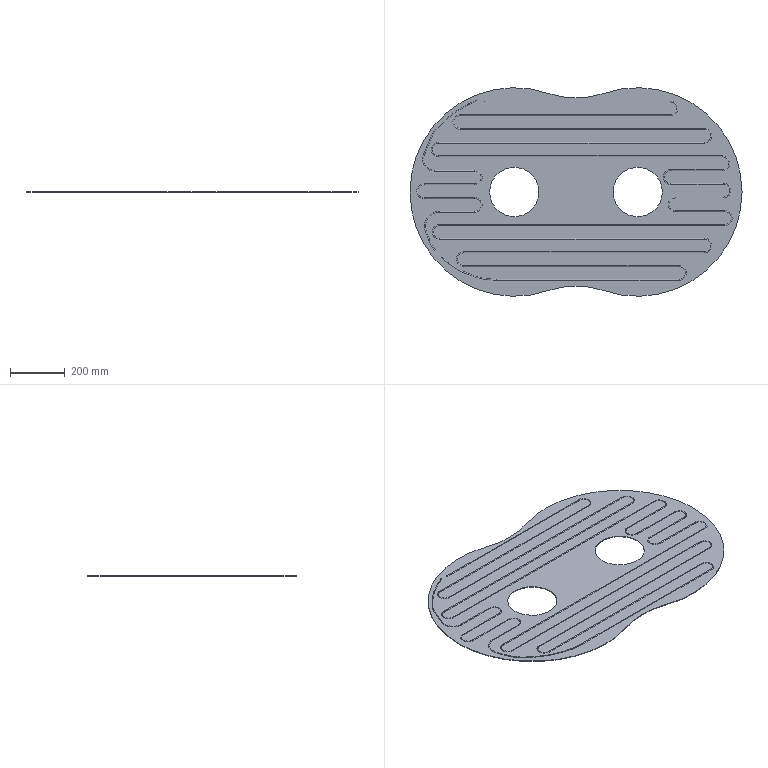Part | NX | 3 solids | 56 faces | box 1210 x 760 x 3.5 mm | volume 1542690 mm3 | cylinder 29 | torus 21 | plane 6 | commonest cylinder face diameters 3 x23 180 x2 640 x2 760 x2
STEP:
#1=CARTESIAN_POINT('',(2647.074,604.738,0.));
#2=VERTEX_POINT('',#1);
#3=CARTESIAN_POINT('',(2647.074,-114.931,0.));
#4=VERTEX_POINT('',#3);
#5=CARTESIAN_POINT('',(2524.931,244.903,0.));
#6=DIRECTION('',(0.,0.,1.));
#7=DIRECTION('',(1.,0.,0.));
#8=AXIS2_PLACEMENT_3D('',#5,#6,#7);
#9=CIRCLE('',#8,380.);
#10=EDGE_CURVE('',#2,#4,#9,.T.);
#11=ORIENTED_EDGE('',*,*,#10,.T.);
#12=CARTESIAN_POINT('',(2647.074,-114.931,2.));
#13=VERTEX_POINT('',#12);
#14=CARTESIAN_POINT('',(2647.074,-114.931,2.));
#15=DIRECTION('',(0.,0.,-1.));
#16=VECTOR('',#15,1.);
#17=LINE('',#14,#16);
#18=EDGE_CURVE('',#13,#4,#17,.T.);
#19=ORIENTED_EDGE('',*,*,#18,.F.);
#20=CARTESIAN_POINT('',(2647.074,604.738,2.));
#21=VERTEX_POINT('',#20);
#22=CARTESIAN_POINT('',(2524.931,244.903,2.));
#23=DIRECTION('',(0.,0.,1.));
#24=DIRECTION('',(1.,0.,0.));
#25=AXIS2_PLACEMENT_3D('',#22,#23,#24);
#26=CIRCLE('',#25,380.);
#27=EDGE_CURVE('',#21,#13,#26,.T.);
#28=ORIENTED_EDGE('',*,*,#27,.F.);
#29=CARTESIAN_POINT('',(2647.074,604.738,2.));
#30=DIRECTION('',(0.,0.,-1.));
#31=VECTOR('',#30,1.);
#32=LINE('',#29,#31);
#33=EDGE_CURVE('',#21,#2,#32,.T.);
#34=ORIENTED_EDGE('',*,*,#33,.T.);
#35=EDGE_LOOP('',(#11,#19,#28,#34));
#36=FACE_OUTER_BOUND('',#35,.T.);
#37=CARTESIAN_POINT('',(2524.931,244.903,2.));
#38=DIRECTION('',(0.,0.,-1.));
#39=DIRECTION('',(-1.,0.,0.));
#40=AXIS2_PLACEMENT_3D('',#37,#38,#39);
#41=CYLINDRICAL_SURFACE('',#40,380.);
#42=ADVANCED_FACE('',(#36),#41,.T.);
#43=CARTESIAN_POINT('',(2852.788,-114.931,0.));
#44=VERTEX_POINT('',#43);
#45=CARTESIAN_POINT('',(2749.931,-417.95,0.));
#46=DIRECTION('',(0.,0.,-1.));
#47=DIRECTION('',(1.,0.,0.));
#48=AXIS2_PLACEMENT_3D('',#45,#46,#47);
#49=CIRCLE('',#48,320.);
#50=EDGE_CURVE('',#4,#44,#49,.T.);
#51=ORIENTED_EDGE('',*,*,#50,.T.);
#52=CARTESIAN_POINT('',(2852.788,-114.931,2.));
#53=VERTEX_POINT('',#52);
#54=CARTESIAN_POINT('',(2852.788,-114.931,2.));
#55=DIRECTION('',(0.,0.,-1.));
#56=VECTOR('',#55,1.);
#57=LINE('',#54,#56);
#58=EDGE_CURVE('',#53,#44,#57,.T.);
#59=ORIENTED_EDGE('',*,*,#58,.F.);
#60=CARTESIAN_POINT('',(2749.931,-417.95,2.));
#61=DIRECTION('',(0.,0.,-1.));
#62=DIRECTION('',(1.,0.,0.));
#63=AXIS2_PLACEMENT_3D('',#60,#61,#62);
#64=CIRCLE('',#63,320.);
#65=EDGE_CURVE('',#13,#53,#64,.T.);
#66=ORIENTED_EDGE('',*,*,#65,.F.);
#67=ORIENTED_EDGE('',*,*,#18,.T.);
#68=EDGE_LOOP('',(#51,#59,#66,#67));
#69=FACE_OUTER_BOUND('',#68,.T.);
#70=CARTESIAN_POINT('',(2749.931,-417.95,2.));
#71=DIRECTION('',(0.,0.,-1.));
#72=DIRECTION('',(-1.,0.,0.));
#73=AXIS2_PLACEMENT_3D('',#70,#71,#72);
#74=CYLINDRICAL_SURFACE('',#73,320.);
#75=ADVANCED_FACE('',(#69),#74,.F.);
#76=CARTESIAN_POINT('',(2852.788,604.738,0.));
#77=VERTEX_POINT('',#76);
#78=CARTESIAN_POINT('',(2974.931,244.903,0.));
#79=DIRECTION('',(0.,0.,1.));
#80=DIRECTION('',(1.,0.,0.));
#81=AXIS2_PLACEMENT_3D('',#78,#79,#80);
#82=CIRCLE('',#81,380.);
#83=EDGE_CURVE('',#44,#77,#82,.T.);
#84=ORIENTED_EDGE('',*,*,#83,.T.);
#85=CARTESIAN_POINT('',(2852.788,604.738,2.));
#86=VERTEX_POINT('',#85);
#87=CARTESIAN_POINT('',(2852.788,604.738,2.));
#88=DIRECTION('',(0.,0.,-1.));
#89=VECTOR('',#88,1.);
#90=LINE('',#87,#89);
#91=EDGE_CURVE('',#86,#77,#90,.T.);
#92=ORIENTED_EDGE('',*,*,#91,.F.);
#93=CARTESIAN_POINT('',(2974.931,244.903,2.));
#94=DIRECTION('',(0.,0.,1.));
#95=DIRECTION('',(1.,0.,0.));
#96=AXIS2_PLACEMENT_3D('',#93,#94,#95);
#97=CIRCLE('',#96,380.);
#98=EDGE_CURVE('',#53,#86,#97,.T.);
#99=ORIENTED_EDGE('',*,*,#98,.F.);
#100=ORIENTED_EDGE('',*,*,#58,.T.);
#101=EDGE_LOOP('',(#84,#92,#99,#100));
#102=FACE_OUTER_BOUND('',#101,.T.);
#103=CARTESIAN_POINT('',(2974.931,244.903,2.));
#104=DIRECTION('',(0.,0.,-1.));
#105=DIRECTION('',(-1.,0.,0.));
#106=AXIS2_PLACEMENT_3D('',#103,#104,#105);
#107=CYLINDRICAL_SURFACE('',#106,380.);
#108=ADVANCED_FACE('',(#102),#107,.T.);
#109=CARTESIAN_POINT('',(2614.931,244.903,2.));
#110=VERTEX_POINT('',#109);
#111=CARTESIAN_POINT('',(2524.931,244.903,2.));
#112=DIRECTION('',(0.,0.,1.));
#113=DIRECTION('',(1.,0.,0.));
#114=AXIS2_PLACEMENT_3D('',#111,#112,#113);
#115=CIRCLE('',#114,90.);
#116=EDGE_CURVE('',#110,#110,#115,.T.);
#117=ORIENTED_EDGE('',*,*,#116,.T.);
#118=EDGE_LOOP('',(#117));
#119=FACE_BOUND('',#118,.T.);
#120=CARTESIAN_POINT('',(2614.931,244.903,0.));
#121=VERTEX_POINT('',#120);
#122=CARTESIAN_POINT('',(2524.931,244.903,0.));
#123=DIRECTION('',(0.,0.,1.));
#124=DIRECTION('',(1.,0.,0.));
#125=AXIS2_PLACEMENT_3D('',#122,#123,#124);
#126=CIRCLE('',#125,90.);
#127=EDGE_CURVE('',#121,#121,#126,.T.);
#128=ORIENTED_EDGE('',*,*,#127,.F.);
#129=EDGE_LOOP('',(#128));
#130=FACE_BOUND('',#129,.T.);
#131=CARTESIAN_POINT('',(2524.931,244.903,2.));
#132=DIRECTION('',(0.,0.,-1.));
#133=DIRECTION('',(-1.,0.,0.));
#134=AXIS2_PLACEMENT_3D('',#131,#132,#133);
#135=CYLINDRICAL_SURFACE('',#134,90.);
#136=ADVANCED_FACE('',(#119,#130),#135,.F.);
#137=CARTESIAN_POINT('',(2749.931,907.757,0.));
#138=DIRECTION('',(0.,0.,-1.));
#139=DIRECTION('',(1.,0.,0.));
#140=AXIS2_PLACEMENT_3D('',#137,#138,#139);
#141=CIRCLE('',#140,320.);
#142=EDGE_CURVE('',#77,#2,#141,.T.);
#143=ORIENTED_EDGE('',*,*,#142,.T.);
#144=ORIENTED_EDGE('',*,*,#33,.F.);
#145=CARTESIAN_POINT('',(2749.931,907.757,2.));
#146=DIRECTION('',(0.,0.,-1.));
#147=DIRECTION('',(1.,0.,0.));
#148=AXIS2_PLACEMENT_3D('',#145,#146,#147);
#149=CIRCLE('',#148,320.);
#150=EDGE_CURVE('',#86,#21,#149,.T.);
#151=ORIENTED_EDGE('',*,*,#150,.F.);
#152=ORIENTED_EDGE('',*,*,#91,.T.);
#153=EDGE_LOOP('',(#143,#144,#151,#152));
#154=FACE_OUTER_BOUND('',#153,.T.);
#155=CARTESIAN_POINT('',(2749.931,907.757,2.));
#156=DIRECTION('',(0.,0.,-1.));
#157=DIRECTION('',(-1.,0.,0.));
#158=AXIS2_PLACEMENT_3D('',#155,#156,#157);
#159=CYLINDRICAL_SURFACE('',#158,320.);
#160=ADVANCED_FACE('',(#154),#159,.F.);
#161=CARTESIAN_POINT('',(3064.931,244.903,2.));
#162=VERTEX_POINT('',#161);
#163=CARTESIAN_POINT('',(2974.931,244.903,2.));
#164=DIRECTION('',(0.,0.,1.));
#165=DIRECTION('',(1.,0.,0.));
#166=AXIS2_PLACEMENT_3D('',#163,#164,#165);
#167=CIRCLE('',#166,90.);
#168=EDGE_CURVE('',#162,#162,#167,.T.);
#169=ORIENTED_EDGE('',*,*,#168,.T.);
#170=EDGE_LOOP('',(#169));
#171=FACE_BOUND('',#170,.T.);
#172=CARTESIAN_POINT('',(3064.931,244.903,0.));
#173=VERTEX_POINT('',#172);
#174=CARTESIAN_POINT('',(2974.931,244.903,0.));
#175=DIRECTION('',(0.,0.,1.));
#176=DIRECTION('',(1.,0.,0.));
#177=AXIS2_PLACEMENT_3D('',#174,#175,#176);
#178=CIRCLE('',#177,90.);
#179=EDGE_CURVE('',#173,#173,#178,.T.);
#180=ORIENTED_EDGE('',*,*,#179,.F.);
#181=EDGE_LOOP('',(#180));
#182=FACE_BOUND('',#181,.T.);
#183=CARTESIAN_POINT('',(2974.931,244.903,2.));
#184=DIRECTION('',(0.,0.,-1.));
#185=DIRECTION('',(-1.,0.,0.));
#186=AXIS2_PLACEMENT_3D('',#183,#184,#185);
#187=CYLINDRICAL_SURFACE('',#186,90.);
#188=ADVANCED_FACE('',(#171,#182),#187,.F.);
#189=ORIENTED_EDGE('',*,*,#27,.T.);
#190=ORIENTED_EDGE('',*,*,#65,.T.);
#191=ORIENTED_EDGE('',*,*,#98,.T.);
#192=ORIENTED_EDGE('',*,*,#150,.T.);
#193=EDGE_LOOP('',(#189,#190,#191,#192));
#194=FACE_BOUND('',#193,.T.);
#195=ORIENTED_EDGE('',*,*,#116,.F.);
#196=EDGE_LOOP('',(#195));
#197=FACE_BOUND('',#196,.T.);
#198=ORIENTED_EDGE('',*,*,#168,.F.);
#199=EDGE_LOOP('',(#198));
#200=FACE_BOUND('',#199,.T.);
#201=CARTESIAN_POINT('',(2637.431,-86.523,2.));
#202=DIRECTION('',(0.,0.,1.));
#203=DIRECTION('',(1.,0.,0.));
#204=AXIS2_PLACEMENT_3D('',#201,#202,#203);
#205=PLANE('',#204);
#206=ADVANCED_FACE('',(#194,#197,#200),#205,.T.);
#207=ORIENTED_EDGE('',*,*,#10,.F.);
#208=ORIENTED_EDGE('',*,*,#142,.F.);
#209=ORIENTED_EDGE('',*,*,#83,.F.);
#210=ORIENTED_EDGE('',*,*,#50,.F.);
#211=EDGE_LOOP('',(#207,#208,#209,#210));
#212=FACE_BOUND('',#211,.T.);
#213=ORIENTED_EDGE('',*,*,#127,.T.);
#214=EDGE_LOOP('',(#213));
#215=FACE_BOUND('',#214,.T.);
#216=ORIENTED_EDGE('',*,*,#179,.T.);
#217=EDGE_LOOP('',(#216));
#218=FACE_BOUND('',#217,.T.);
#219=CARTESIAN_POINT('',(2637.431,-86.523,0.));
#220=DIRECTION('',(0.,0.,1.));
#221=DIRECTION('',(1.,0.,0.));
#222=AXIS2_PLACEMENT_3D('',#219,#220,#221);
#223=PLANE('',#222);
#224=ADVANCED_FACE('',(#212,#215,#218),#223,.F.);
#225=CLOSED_SHELL('',(#42,#75,#108,#136,#160,#188,#206,#224));
#226=MANIFOLD_SOLID_BREP('',#225);
#227=CARTESIAN_POINT('',(2239.156,471.609,2.));
#228=VERTEX_POINT('',#227);
#229=CARTESIAN_POINT('',(2238.018,472.586,2.));
#230=DIRECTION('',(-0.6509,-0.7592,0.));
#231=DIRECTION('',(0.7592,-0.6509,0.));
#232=AXIS2_PLACEMENT_3D('',#229,#230,#231);
#233=CIRCLE('',#232,1.5);
#234=EDGE_CURVE('',#228,#228,#233,.T.);
#235=ORIENTED_EDGE('',*,*,#234,.T.);
#236=EDGE_LOOP('',(#235));
#237=FACE_BOUND('',#236,.T.);
#238=CARTESIAN_POINT('',(2232.864,464.27,2.));
#239=VERTEX_POINT('',#238);
#240=CARTESIAN_POINT('',(2231.725,465.246,2.));
#241=DIRECTION('',(-0.6509,-0.7592,0.));
#242=DIRECTION('',(0.7592,-0.6509,0.));
#243=AXIS2_PLACEMENT_3D('',#240,#241,#242);
#244=CIRCLE('',#243,1.5);
#245=EDGE_CURVE('',#239,#239,#244,.T.);
#246=ORIENTED_EDGE('',*,*,#245,.F.);
#247=EDGE_LOOP('',(#246));
#248=FACE_BOUND('',#247,.T.);
#249=CARTESIAN_POINT('',(2238.018,472.586,2.));
#250=DIRECTION('',(-0.6509,-0.7592,0.));
#251=DIRECTION('',(0.7592,-0.6509,0.));
#252=AXIS2_PLACEMENT_3D('',#249,#250,#251);
#253=CYLINDRICAL_SURFACE('',#252,1.5);
#254=ADVANCED_FACE('',(#237,#248),#253,.T.);
#255=CARTESIAN_POINT('',(2359.815,563.182,2.));
#256=VERTEX_POINT('',#255);
#257=CARTESIAN_POINT('',(2359.181,564.541,2.));
#258=DIRECTION('',(-0.9063,-0.4226,0.));
#259=DIRECTION('',(0.4226,-0.9063,0.));
#260=AXIS2_PLACEMENT_3D('',#257,#258,#259);
#261=CIRCLE('',#260,1.5);
#262=EDGE_CURVE('',#256,#256,#261,.T.);
#263=ORIENTED_EDGE('',*,*,#262,.T.);
#264=EDGE_LOOP('',(#263));
#265=FACE_BOUND('',#264,.T.);
#266=ORIENTED_EDGE('',*,*,#234,.F.);
#267=EDGE_LOOP('',(#266));
#268=FACE_BOUND('',#267,.T.);
#269=CARTESIAN_POINT('',(2511.324,238.271,2.));
#270=DIRECTION('',(0.,0.,1.));
#271=DIRECTION('',(1.,0.,0.));
#272=AXIS2_PLACEMENT_3D('',#269,#270,#271);
#273=TOROIDAL_SURFACE('',#272,360.,1.5);
#274=ADVANCED_FACE('',(#265,#268),#273,.T.);
#275=ORIENTED_EDGE('',*,*,#262,.F.);
#276=EDGE_LOOP('',(#275));
#277=FACE_BOUND('',#276,.T.);
#278=CARTESIAN_POINT('',(2388.99,576.786,2.));
#279=VERTEX_POINT('',#278);
#280=CARTESIAN_POINT('',(2388.356,578.146,2.));
#281=DIRECTION('',(-0.9063,-0.4226,0.));
#282=DIRECTION('',(0.4226,-0.9063,0.));
#283=AXIS2_PLACEMENT_3D('',#280,#281,#282);
#284=CIRCLE('',#283,1.5);
#285=EDGE_CURVE('',#279,#279,#284,.T.);
#286=ORIENTED_EDGE('',*,*,#285,.T.);
#287=EDGE_LOOP('',(#286));
#288=FACE_BOUND('',#287,.T.);
#289=CARTESIAN_POINT('',(2359.181,564.541,2.));
#290=DIRECTION('',(0.9063,0.4226,0.));
#291=DIRECTION('',(-0.4226,0.9063,0.));
#292=AXIS2_PLACEMENT_3D('',#289,#290,#291);
#293=CYLINDRICAL_SURFACE('',#292,1.5);
#294=ADVANCED_FACE('',(#277,#288),#293,.T.);
#295=ORIENTED_EDGE('',*,*,#245,.T.);
#296=EDGE_LOOP('',(#295));
#297=FACE_OUTER_BOUND('',#296,.T.);
#298=CARTESIAN_POINT('',(2231.725,465.246,2.));
#299=DIRECTION('',(-0.6509,-0.7592,0.));
#300=DIRECTION('',(0.7592,-0.6509,0.));
#301=AXIS2_PLACEMENT_3D('',#298,#299,#300);
#302=PLANE('',#301);
#303=ADVANCED_FACE('',(#297),#302,.T.);
#304=ORIENTED_EDGE('',*,*,#285,.F.);
#305=EDGE_LOOP('',(#304));
#306=FACE_OUTER_BOUND('',#305,.T.);
#307=CARTESIAN_POINT('',(2388.356,578.146,2.));
#308=DIRECTION('',(-0.9063,-0.4226,0.));
#309=DIRECTION('',(0.4226,-0.9063,0.));
#310=AXIS2_PLACEMENT_3D('',#307,#308,#309);
#311=PLANE('',#310);
#312=ADVANCED_FACE('',(#306),#311,.F.);
#313=CLOSED_SHELL('',(#254,#274,#294,#303,#312));
#314=MANIFOLD_SOLID_BREP('',#313);
#315=CARTESIAN_POINT('',(3094.34,573.238,2.));
#316=VERTEX_POINT('',#315);
#317=CARTESIAN_POINT('',(3094.34,574.738,2.));
#318=DIRECTION('',(-1.,0.,0.));
#319=DIRECTION('',(0.,-1.,0.));
#320=AXIS2_PLACEMENT_3D('',#317,#318,#319);
#321=CIRCLE('',#320,1.5);
#322=EDGE_CURVE('',#316,#316,#321,.T.);
#323=ORIENTED_EDGE('',*,*,#322,.T.);
#324=EDGE_LOOP('',(#323));
#325=FACE_BOUND('',#324,.T.);
#326=CARTESIAN_POINT('',(2415.256,573.238,2.));
#327=VERTEX_POINT('',#326);
#328=CARTESIAN_POINT('',(2415.256,574.738,2.));
#329=DIRECTION('',(-1.,0.,0.));
#330=DIRECTION('',(0.,-1.,0.));
#331=AXIS2_PLACEMENT_3D('',#328,#329,#330);
#332=CIRCLE('',#331,1.5);
#333=EDGE_CURVE('',#327,#327,#332,.T.);
#334=ORIENTED_EDGE('',*,*,#333,.F.);
#335=EDGE_LOOP('',(#334));
#336=FACE_BOUND('',#335,.T.);
#337=CARTESIAN_POINT('',(3094.34,574.738,2.));
#338=DIRECTION('',(-1.,0.,0.));
#339=DIRECTION('',(0.,0.,1.));
#340=AXIS2_PLACEMENT_3D('',#337,#338,#339);
#341=CYLINDRICAL_SURFACE('',#340,1.5);
#342=ADVANCED_FACE('',(#325,#336),#341,.T.);
#343=CARTESIAN_POINT('',(3094.34,526.238,2.));
#344=VERTEX_POINT('',#343);
#345=CARTESIAN_POINT('',(3094.34,524.738,2.));
#346=DIRECTION('',(1.,0.,0.));
#347=DIRECTION('',(0.,1.,0.));
#348=AXIS2_PLACEMENT_3D('',#345,#346,#347);
#349=CIRCLE('',#348,1.5);
#350=EDGE_CURVE('',#344,#344,#349,.T.);
#351=ORIENTED_EDGE('',*,*,#350,.T.);
#352=EDGE_LOOP('',(#351));
#353=FACE_BOUND('',#352,.T.);
#354=ORIENTED_EDGE('',*,*,#322,.F.);
#355=EDGE_LOOP('',(#354));
#356=FACE_BOUND('',#355,.T.);
#357=CARTESIAN_POINT('',(3094.34,549.738,2.));
#358=DIRECTION('',(0.,0.,1.));
#359=DIRECTION('',(1.,0.,0.));
#360=AXIS2_PLACEMENT_3D('',#357,#358,#359);
#361=TOROIDAL_SURFACE('',#360,25.,1.5);
#362=ADVANCED_FACE('',(#353,#356),#361,.T.);
#363=CARTESIAN_POINT('',(2327.943,526.238,2.));
#364=VERTEX_POINT('',#363);
#365=CARTESIAN_POINT('',(2327.943,524.738,2.));
#366=DIRECTION('',(1.,0.,0.));
#367=DIRECTION('',(0.,1.,0.));
#368=AXIS2_PLACEMENT_3D('',#365,#366,#367);
#369=CIRCLE('',#368,1.5);
#370=EDGE_CURVE('',#364,#364,#369,.T.);
#371=ORIENTED_EDGE('',*,*,#370,.T.);
#372=EDGE_LOOP('',(#371));
#373=FACE_BOUND('',#372,.T.);
#374=ORIENTED_EDGE('',*,*,#350,.F.);
#375=EDGE_LOOP('',(#374));
#376=FACE_BOUND('',#375,.T.);
#377=CARTESIAN_POINT('',(2327.943,524.738,2.));
#378=DIRECTION('',(1.,0.,0.));
#379=DIRECTION('',(0.,1.,0.));
#380=AXIS2_PLACEMENT_3D('',#377,#378,#379);
#381=CYLINDRICAL_SURFACE('',#380,1.5);
#382=ADVANCED_FACE('',(#373,#376),#381,.T.);
#383=CARTESIAN_POINT('',(2327.943,473.238,2.));
#384=VERTEX_POINT('',#383);
#385=CARTESIAN_POINT('',(2327.943,474.738,2.));
#386=DIRECTION('',(-1.,0.,0.));
#387=DIRECTION('',(0.,-1.,0.));
#388=AXIS2_PLACEMENT_3D('',#385,#386,#387);
#389=CIRCLE('',#388,1.5);
#390=EDGE_CURVE('',#384,#384,#389,.T.);
#391=ORIENTED_EDGE('',*,*,#390,.T.);
#392=EDGE_LOOP('',(#391));
#393=FACE_BOUND('',#392,.T.);
#394=ORIENTED_EDGE('',*,*,#370,.F.);
#395=EDGE_LOOP('',(#394));
#396=FACE_BOUND('',#395,.T.);
#397=CARTESIAN_POINT('',(2327.943,499.738,2.));
#398=DIRECTION('',(0.,0.,-1.));
#399=DIRECTION('',(-1.,0.,0.));
#400=AXIS2_PLACEMENT_3D('',#397,#398,#399);
#401=TOROIDAL_SURFACE('',#400,25.,1.5);
#402=ADVANCED_FACE('',(#393,#396),#401,.T.);
#403=CARTESIAN_POINT('',(3217.854,473.238,2.));
#404=VERTEX_POINT('',#403);
#405=CARTESIAN_POINT('',(3217.854,474.738,2.));
#406=DIRECTION('',(-1.,0.,0.));
#407=DIRECTION('',(0.,-1.,0.));
#408=AXIS2_PLACEMENT_3D('',#405,#406,#407);
#409=CIRCLE('',#408,1.5);
#410=EDGE_CURVE('',#404,#404,#409,.T.);
#411=ORIENTED_EDGE('',*,*,#410,.T.);
#412=EDGE_LOOP('',(#411));
#413=FACE_BOUND('',#412,.T.);
#414=ORIENTED_EDGE('',*,*,#390,.F.);
#415=EDGE_LOOP('',(#414));
#416=FACE_BOUND('',#415,.T.);
#417=CARTESIAN_POINT('',(3217.854,474.738,2.));
#418=DIRECTION('',(-1.,0.,0.));
#419=DIRECTION('',(0.,0.,1.));
#420=AXIS2_PLACEMENT_3D('',#417,#418,#419);
#421=CYLINDRICAL_SURFACE('',#420,1.5);
#422=ADVANCED_FACE('',(#413,#416),#421,.T.);
#423=CARTESIAN_POINT('',(3217.854,426.238,2.));
#424=VERTEX_POINT('',#423);
#425=CARTESIAN_POINT('',(3217.854,424.738,2.));
#426=DIRECTION('',(1.,0.,0.));
#427=DIRECTION('',(0.,1.,0.));
#428=AXIS2_PLACEMENT_3D('',#425,#426,#427);
#429=CIRCLE('',#428,1.5);
#430=EDGE_CURVE('',#424,#424,#429,.T.);
#431=ORIENTED_EDGE('',*,*,#430,.T.);
#432=EDGE_LOOP('',(#431));
#433=FACE_BOUND('',#432,.T.);
#434=ORIENTED_EDGE('',*,*,#410,.F.);
#435=EDGE_LOOP('',(#434));
#436=FACE_BOUND('',#435,.T.);
#437=CARTESIAN_POINT('',(3217.854,449.738,2.));
#438=DIRECTION('',(0.,0.,1.));
#439=DIRECTION('',(1.,0.,0.));
#440=AXIS2_PLACEMENT_3D('',#437,#438,#439);
#441=TOROIDAL_SURFACE('',#440,25.,1.5);
#442=ADVANCED_FACE('',(#433,#436),#441,.T.);
#443=CARTESIAN_POINT('',(2248.791,426.238,2.));
#444=VERTEX_POINT('',#443);
#445=CARTESIAN_POINT('',(2248.791,424.738,2.));
#446=DIRECTION('',(1.,0.,0.));
#447=DIRECTION('',(0.,1.,0.));
#448=AXIS2_PLACEMENT_3D('',#445,#446,#447);
#449=CIRCLE('',#448,1.5);
#450=EDGE_CURVE('',#444,#444,#449,.T.);
#451=ORIENTED_EDGE('',*,*,#450,.T.);
#452=EDGE_LOOP('',(#451));
#453=FACE_BOUND('',#452,.T.);
#454=ORIENTED_EDGE('',*,*,#430,.F.);
#455=EDGE_LOOP('',(#454));
#456=FACE_BOUND('',#455,.T.);
#457=CARTESIAN_POINT('',(2248.791,424.738,2.));
#458=DIRECTION('',(1.,0.,0.));
#459=DIRECTION('',(0.,1.,0.));
#460=AXIS2_PLACEMENT_3D('',#457,#458,#459);
#461=CYLINDRICAL_SURFACE('',#460,1.5);
#462=ADVANCED_FACE('',(#453,#456),#461,.T.);
#463=CARTESIAN_POINT('',(2248.791,373.238,2.));
#464=VERTEX_POINT('',#463);
#465=CARTESIAN_POINT('',(2248.791,374.738,2.));
#466=DIRECTION('',(-1.,0.,0.));
#467=DIRECTION('',(0.,-1.,0.));
#468=AXIS2_PLACEMENT_3D('',#465,#466,#467);
#469=CIRCLE('',#468,1.5);
#470=EDGE_CURVE('',#464,#464,#469,.T.);
#471=ORIENTED_EDGE('',*,*,#470,.T.);
#472=EDGE_LOOP('',(#471));
#473=FACE_BOUND('',#472,.T.);
#474=ORIENTED_EDGE('',*,*,#450,.F.);
#475=EDGE_LOOP('',(#474));
#476=FACE_BOUND('',#475,.T.);
#477=CARTESIAN_POINT('',(2248.791,399.738,2.));
#478=DIRECTION('',(0.,0.,-1.));
#479=DIRECTION('',(-1.,0.,0.));
#480=AXIS2_PLACEMENT_3D('',#477,#478,#479);
#481=TOROIDAL_SURFACE('',#480,25.,1.5);
#482=ADVANCED_FACE('',(#473,#476),#481,.T.);
#483=CARTESIAN_POINT('',(3283.473,373.238,2.));
#484=VERTEX_POINT('',#483);
#485=CARTESIAN_POINT('',(3283.473,374.738,2.));
#486=DIRECTION('',(-1.,0.,0.));
#487=DIRECTION('',(0.,-1.,0.));
#488=AXIS2_PLACEMENT_3D('',#485,#486,#487);
#489=CIRCLE('',#488,1.5);
#490=EDGE_CURVE('',#484,#484,#489,.T.);
#491=ORIENTED_EDGE('',*,*,#490,.T.);
#492=EDGE_LOOP('',(#491));
#493=FACE_BOUND('',#492,.T.);
#494=ORIENTED_EDGE('',*,*,#470,.F.);
#495=EDGE_LOOP('',(#494));
#496=FACE_BOUND('',#495,.T.);
#497=CARTESIAN_POINT('',(3283.473,374.738,2.));
#498=DIRECTION('',(-1.,0.,0.));
#499=DIRECTION('',(0.,0.,1.));
#500=AXIS2_PLACEMENT_3D('',#497,#498,#499);
#501=CYLINDRICAL_SURFACE('',#500,1.5);
#502=ADVANCED_FACE('',(#493,#496),#501,.T.);
#503=CARTESIAN_POINT('',(3283.473,326.238,2.));
#504=VERTEX_POINT('',#503);
#505=CARTESIAN_POINT('',(3283.473,324.738,2.));
#506=DIRECTION('',(1.,0.,0.));
#507=DIRECTION('',(0.,1.,0.));
#508=AXIS2_PLACEMENT_3D('',#505,#506,#507);
#509=CIRCLE('',#508,1.5);
#510=EDGE_CURVE('',#504,#504,#509,.T.);
#511=ORIENTED_EDGE('',*,*,#510,.T.);
#512=EDGE_LOOP('',(#511));
#513=FACE_BOUND('',#512,.T.);
#514=ORIENTED_EDGE('',*,*,#490,.F.);
#515=EDGE_LOOP('',(#514));
#516=FACE_BOUND('',#515,.T.);
#517=CARTESIAN_POINT('',(3283.473,349.738,2.));
#518=DIRECTION('',(0.,0.,1.));
#519=DIRECTION('',(1.,0.,0.));
#520=AXIS2_PLACEMENT_3D('',#517,#518,#519);
#521=TOROIDAL_SURFACE('',#520,25.,1.5);
#522=ADVANCED_FACE('',(#513,#516),#521,.T.);
#523=CARTESIAN_POINT('',(3094.801,326.238,2.));
#524=VERTEX_POINT('',#523);
#525=CARTESIAN_POINT('',(3094.801,324.738,2.));
#526=DIRECTION('',(1.,0.,0.));
#527=DIRECTION('',(0.,1.,0.));
#528=AXIS2_PLACEMENT_3D('',#525,#526,#527);
#529=CIRCLE('',#528,1.5);
#530=EDGE_CURVE('',#524,#524,#529,.T.);
#531=ORIENTED_EDGE('',*,*,#530,.T.);
#532=EDGE_LOOP('',(#531));
#533=FACE_BOUND('',#532,.T.);
#534=ORIENTED_EDGE('',*,*,#510,.F.);
#535=EDGE_LOOP('',(#534));
#536=FACE_BOUND('',#535,.T.);
#537=CARTESIAN_POINT('',(3094.801,324.738,2.));
#538=DIRECTION('',(1.,0.,0.));
#539=DIRECTION('',(0.,0.,-1.));
#540=AXIS2_PLACEMENT_3D('',#537,#538,#539);
#541=CYLINDRICAL_SURFACE('',#540,1.5);
#542=ADVANCED_FACE('',(#533,#536),#541,.T.);
#543=CARTESIAN_POINT('',(3094.801,273.238,2.));
#544=VERTEX_POINT('',#543);
#545=CARTESIAN_POINT('',(3094.801,274.738,2.));
#546=DIRECTION('',(-1.,0.,0.));
#547=DIRECTION('',(0.,-1.,0.));
#548=AXIS2_PLACEMENT_3D('',#545,#546,#547);
#549=CIRCLE('',#548,1.5);
#550=EDGE_CURVE('',#544,#544,#549,.T.);
#551=ORIENTED_EDGE('',*,*,#550,.T.);
#552=EDGE_LOOP('',(#551));
#553=FACE_BOUND('',#552,.T.);
#554=ORIENTED_EDGE('',*,*,#530,.F.);
#555=EDGE_LOOP('',(#554));
#556=FACE_BOUND('',#555,.T.);
#557=CARTESIAN_POINT('',(3094.801,299.738,2.));
#558=DIRECTION('',(0.,0.,-1.));
#559=DIRECTION('',(-1.,0.,0.));
#560=AXIS2_PLACEMENT_3D('',#557,#558,#559);
#561=TOROIDAL_SURFACE('',#560,25.,1.5);
#562=ADVANCED_FACE('',(#553,#556),#561,.T.);
#563=CARTESIAN_POINT('',(3286.978,273.238,2.));
#564=VERTEX_POINT('',#563);
#565=CARTESIAN_POINT('',(3286.978,274.738,2.));
#566=DIRECTION('',(-1.,0.,0.));
#567=DIRECTION('',(0.,-1.,0.));
#568=AXIS2_PLACEMENT_3D('',#565,#566,#567);
#569=CIRCLE('',#568,1.5);
#570=EDGE_CURVE('',#564,#564,#569,.T.);
#571=ORIENTED_EDGE('',*,*,#570,.T.);
#572=EDGE_LOOP('',(#571));
#573=FACE_BOUND('',#572,.T.);
#574=ORIENTED_EDGE('',*,*,#550,.F.);
#575=EDGE_LOOP('',(#574));
#576=FACE_BOUND('',#575,.T.);
#577=CARTESIAN_POINT('',(3286.978,274.738,2.));
#578=DIRECTION('',(-1.,0.,0.));
#579=DIRECTION('',(0.,-1.,0.));
#580=AXIS2_PLACEMENT_3D('',#577,#578,#579);
#581=CYLINDRICAL_SURFACE('',#580,1.5);
#582=ADVANCED_FACE('',(#573,#576),#581,.T.);
#583=CARTESIAN_POINT('',(3286.978,226.238,2.));
#584=VERTEX_POINT('',#583);
#585=CARTESIAN_POINT('',(3286.978,224.738,2.));
#586=DIRECTION('',(1.,0.,0.));
#587=DIRECTION('',(0.,1.,0.));
#588=AXIS2_PLACEMENT_3D('',#585,#586,#587);
#589=CIRCLE('',#588,1.5);
#590=EDGE_CURVE('',#584,#584,#589,.T.);
#591=ORIENTED_EDGE('',*,*,#590,.T.);
#592=EDGE_LOOP('',(#591));
#593=FACE_BOUND('',#592,.T.);
#594=ORIENTED_EDGE('',*,*,#570,.F.);
#595=EDGE_LOOP('',(#594));
#596=FACE_BOUND('',#595,.T.);
#597=CARTESIAN_POINT('',(3286.978,249.738,2.));
#598=DIRECTION('',(0.,0.,1.));
#599=DIRECTION('',(1.,0.,0.));
#600=AXIS2_PLACEMENT_3D('',#597,#598,#599);
#601=TOROIDAL_SURFACE('',#600,25.,1.5);
#602=ADVANCED_FACE('',(#593,#596),#601,.T.);
#603=CARTESIAN_POINT('',(3112.108,226.238,2.));
#604=VERTEX_POINT('',#603);
#605=CARTESIAN_POINT('',(3112.108,224.738,2.));
#606=DIRECTION('',(1.,0.,0.));
#607=DIRECTION('',(0.,1.,0.));
#608=AXIS2_PLACEMENT_3D('',#605,#606,#607);
#609=CIRCLE('',#608,1.5);
#610=EDGE_CURVE('',#604,#604,#609,.T.);
#611=ORIENTED_EDGE('',*,*,#610,.T.);
#612=EDGE_LOOP('',(#611));
#613=FACE_BOUND('',#612,.T.);
#614=ORIENTED_EDGE('',*,*,#590,.F.);
#615=EDGE_LOOP('',(#614));
#616=FACE_BOUND('',#615,.T.);
#617=CARTESIAN_POINT('',(3112.108,224.738,2.));
#618=DIRECTION('',(1.,0.,0.));
#619=DIRECTION('',(0.,1.,0.));
#620=AXIS2_PLACEMENT_3D('',#617,#618,#619);
#621=CYLINDRICAL_SURFACE('',#620,1.5);
#622=ADVANCED_FACE('',(#613,#616),#621,.T.);
#623=CARTESIAN_POINT('',(3112.108,173.238,2.));
#624=VERTEX_POINT('',#623);
#625=CARTESIAN_POINT('',(3112.108,174.738,2.));
#626=DIRECTION('',(-1.,0.,0.));
#627=DIRECTION('',(0.,-1.,0.));
#628=AXIS2_PLACEMENT_3D('',#625,#626,#627);
#629=CIRCLE('',#628,1.5);
#630=EDGE_CURVE('',#624,#624,#629,.T.);
#631=ORIENTED_EDGE('',*,*,#630,.T.);
#632=EDGE_LOOP('',(#631));
#633=FACE_BOUND('',#632,.T.);
#634=ORIENTED_EDGE('',*,*,#610,.F.);
#635=EDGE_LOOP('',(#634));
#636=FACE_BOUND('',#635,.T.);
#637=CARTESIAN_POINT('',(3112.108,199.738,2.));
#638=DIRECTION('',(0.,0.,-1.));
#639=DIRECTION('',(-1.,0.,0.));
#640=AXIS2_PLACEMENT_3D('',#637,#638,#639);
#641=TOROIDAL_SURFACE('',#640,25.,1.5);
#642=ADVANCED_FACE('',(#633,#636),#641,.T.);
#643=CARTESIAN_POINT('',(3292.679,173.238,2.));
#644=VERTEX_POINT('',#643);
#645=CARTESIAN_POINT('',(3292.679,174.738,2.));
#646=DIRECTION('',(-1.,0.,0.));
#647=DIRECTION('',(0.,-1.,0.));
#648=AXIS2_PLACEMENT_3D('',#645,#646,#647);
#649=CIRCLE('',#648,1.5);
#650=EDGE_CURVE('',#644,#644,#649,.T.);
#651=ORIENTED_EDGE('',*,*,#650,.T.);
#652=EDGE_LOOP('',(#651));
#653=FACE_BOUND('',#652,.T.);
#654=ORIENTED_EDGE('',*,*,#630,.F.);
#655=EDGE_LOOP('',(#654));
#656=FACE_BOUND('',#655,.T.);
#657=CARTESIAN_POINT('',(3292.679,174.738,2.));
#658=DIRECTION('',(-1.,0.,0.));
#659=DIRECTION('',(0.,0.,1.));
#660=AXIS2_PLACEMENT_3D('',#657,#658,#659);
#661=CYLINDRICAL_SURFACE('',#660,1.5);
#662=ADVANCED_FACE('',(#653,#656),#661,.T.);
#663=CARTESIAN_POINT('',(3292.679,126.238,2.));
#664=VERTEX_POINT('',#663);
#665=CARTESIAN_POINT('',(3292.679,124.738,2.));
#666=DIRECTION('',(1.,0.,0.));
#667=DIRECTION('',(0.,1.,0.));
#668=AXIS2_PLACEMENT_3D('',#665,#666,#667);
#669=CIRCLE('',#668,1.5);
#670=EDGE_CURVE('',#664,#664,#669,.T.);
#671=ORIENTED_EDGE('',*,*,#670,.T.);
#672=EDGE_LOOP('',(#671));
#673=FACE_BOUND('',#672,.T.);
#674=ORIENTED_EDGE('',*,*,#650,.F.);
#675=EDGE_LOOP('',(#674));
#676=FACE_BOUND('',#675,.T.);
#677=CARTESIAN_POINT('',(3292.679,149.738,2.));
#678=DIRECTION('',(0.,0.,1.));
#679=DIRECTION('',(1.,0.,0.));
#680=AXIS2_PLACEMENT_3D('',#677,#678,#679);
#681=TOROIDAL_SURFACE('',#680,25.,1.5);
#682=ADVANCED_FACE('',(#673,#676),#681,.T.);
#683=CARTESIAN_POINT('',(2252.82,126.238,2.));
#684=VERTEX_POINT('',#683);
#685=CARTESIAN_POINT('',(2252.82,124.738,2.));
#686=DIRECTION('',(1.,0.,0.));
#687=DIRECTION('',(0.,1.,0.));
#688=AXIS2_PLACEMENT_3D('',#685,#686,#687);
#689=CIRCLE('',#688,1.5);
#690=EDGE_CURVE('',#684,#684,#689,.T.);
#691=ORIENTED_EDGE('',*,*,#690,.T.);
#692=EDGE_LOOP('',(#691));
#693=FACE_BOUND('',#692,.T.);
#694=ORIENTED_EDGE('',*,*,#670,.F.);
#695=EDGE_LOOP('',(#694));
#696=FACE_BOUND('',#695,.T.);
#697=CARTESIAN_POINT('',(2252.82,124.738,2.));
#698=DIRECTION('',(1.,0.,0.));
#699=DIRECTION('',(0.,1.,0.));
#700=AXIS2_PLACEMENT_3D('',#697,#698,#699);
#701=CYLINDRICAL_SURFACE('',#700,1.5);
#702=ADVANCED_FACE('',(#693,#696),#701,.T.);
#703=CARTESIAN_POINT('',(2252.82,73.238,2.));
#704=VERTEX_POINT('',#703);
#705=CARTESIAN_POINT('',(2252.82,74.738,2.));
#706=DIRECTION('',(-1.,0.,0.));
#707=DIRECTION('',(0.,-1.,0.));
#708=AXIS2_PLACEMENT_3D('',#705,#706,#707);
#709=CIRCLE('',#708,1.5);
#710=EDGE_CURVE('',#704,#704,#709,.T.);
#711=ORIENTED_EDGE('',*,*,#710,.T.);
#712=EDGE_LOOP('',(#711));
#713=FACE_BOUND('',#712,.T.);
#714=ORIENTED_EDGE('',*,*,#690,.F.);
#715=EDGE_LOOP('',(#714));
#716=FACE_BOUND('',#715,.T.);
#717=CARTESIAN_POINT('',(2252.82,99.738,2.));
#718=DIRECTION('',(0.,0.,-1.));
#719=DIRECTION('',(-1.,0.,0.));
#720=AXIS2_PLACEMENT_3D('',#717,#718,#719);
#721=TOROIDAL_SURFACE('',#720,25.,1.5);
#722=ADVANCED_FACE('',(#713,#716),#721,.T.);
#723=CARTESIAN_POINT('',(3217.82,73.238,2.));
#724=VERTEX_POINT('',#723);
#725=CARTESIAN_POINT('',(3217.82,74.738,2.));
#726=DIRECTION('',(-1.,0.,0.));
#727=DIRECTION('',(0.,-1.,0.));
#728=AXIS2_PLACEMENT_3D('',#725,#726,#727);
#729=CIRCLE('',#728,1.5);
#730=EDGE_CURVE('',#724,#724,#729,.T.);
#731=ORIENTED_EDGE('',*,*,#730,.T.);
#732=EDGE_LOOP('',(#731));
#733=FACE_BOUND('',#732,.T.);
#734=ORIENTED_EDGE('',*,*,#710,.F.);
#735=EDGE_LOOP('',(#734));
#736=FACE_BOUND('',#735,.T.);
#737=CARTESIAN_POINT('',(3217.82,74.738,2.));
#738=DIRECTION('',(-1.,0.,0.));
#739=DIRECTION('',(0.,0.,1.));
#740=AXIS2_PLACEMENT_3D('',#737,#738,#739);
#741=CYLINDRICAL_SURFACE('',#740,1.5);
#742=ADVANCED_FACE('',(#733,#736),#741,.T.);
#743=CARTESIAN_POINT('',(3217.82,26.238,2.));
#744=VERTEX_POINT('',#743);
#745=CARTESIAN_POINT('',(3217.82,24.738,2.));
#746=DIRECTION('',(1.,0.,0.));
#747=DIRECTION('',(0.,1.,0.));
#748=AXIS2_PLACEMENT_3D('',#745,#746,#747);
#749=CIRCLE('',#748,1.5);
#750=EDGE_CURVE('',#744,#744,#749,.T.);
#751=ORIENTED_EDGE('',*,*,#750,.T.);
#752=EDGE_LOOP('',(#751));
#753=FACE_BOUND('',#752,.T.);
#754=ORIENTED_EDGE('',*,*,#730,.F.);
#755=EDGE_LOOP('',(#754));
#756=FACE_BOUND('',#755,.T.);
#757=CARTESIAN_POINT('',(3217.82,49.738,2.));
#758=DIRECTION('',(0.,0.,1.));
#759=DIRECTION('',(1.,0.,0.));
#760=AXIS2_PLACEMENT_3D('',#757,#758,#759);
#761=TOROIDAL_SURFACE('',#760,25.,1.5);
#762=ADVANCED_FACE('',(#753,#756),#761,.T.);
#763=CARTESIAN_POINT('',(2340.961,26.238,2.));
#764=VERTEX_POINT('',#763);
#765=CARTESIAN_POINT('',(2340.961,24.738,2.));
#766=DIRECTION('',(1.,0.,0.));
#767=DIRECTION('',(0.,1.,0.));
#768=AXIS2_PLACEMENT_3D('',#765,#766,#767);
#769=CIRCLE('',#768,1.5);
#770=EDGE_CURVE('',#764,#764,#769,.T.);
#771=ORIENTED_EDGE('',*,*,#770,.T.);
#772=EDGE_LOOP('',(#771));
#773=FACE_BOUND('',#772,.T.);
#774=ORIENTED_EDGE('',*,*,#750,.F.);
#775=EDGE_LOOP('',(#774));
#776=FACE_BOUND('',#775,.T.);
#777=CARTESIAN_POINT('',(2340.961,24.738,2.));
#778=DIRECTION('',(1.,0.,0.));
#779=DIRECTION('',(0.,1.,0.));
#780=AXIS2_PLACEMENT_3D('',#777,#778,#779);
#781=CYLINDRICAL_SURFACE('',#780,1.5);
#782=ADVANCED_FACE('',(#773,#776),#781,.T.);
#783=CARTESIAN_POINT('',(2340.961,-26.762,2.));
#784=VERTEX_POINT('',#783);
#785=CARTESIAN_POINT('',(2340.961,-25.262,2.));
#786=DIRECTION('',(-1.,0.,0.));
#787=DIRECTION('',(0.,-1.,0.));
#788=AXIS2_PLACEMENT_3D('',#785,#786,#787);
#789=CIRCLE('',#788,1.5);
#790=EDGE_CURVE('',#784,#784,#789,.T.);
#791=ORIENTED_EDGE('',*,*,#790,.T.);
#792=EDGE_LOOP('',(#791));
#793=FACE_BOUND('',#792,.T.);
#794=ORIENTED_EDGE('',*,*,#770,.F.);
#795=EDGE_LOOP('',(#794));
#796=FACE_BOUND('',#795,.T.);
#797=CARTESIAN_POINT('',(2340.961,-0.2617,2.));
#798=DIRECTION('',(0.,0.,-1.));
#799=DIRECTION('',(-1.,0.,0.));
#800=AXIS2_PLACEMENT_3D('',#797,#798,#799);
#801=TOROIDAL_SURFACE('',#800,25.,1.5);
#802=ADVANCED_FACE('',(#793,#796),#801,.T.);
#803=CARTESIAN_POINT('',(3125.566,-26.762,2.));
#804=VERTEX_POINT('',#803);
#805=CARTESIAN_POINT('',(3125.566,-25.262,2.));
#806=DIRECTION('',(-1.,0.,0.));
#807=DIRECTION('',(0.,-1.,0.));
#808=AXIS2_PLACEMENT_3D('',#805,#806,#807);
#809=CIRCLE('',#808,1.5);
#810=EDGE_CURVE('',#804,#804,#809,.T.);
#811=ORIENTED_EDGE('',*,*,#810,.T.);
#812=EDGE_LOOP('',(#811));
#813=FACE_BOUND('',#812,.T.);
#814=ORIENTED_EDGE('',*,*,#790,.F.);
#815=EDGE_LOOP('',(#814));
#816=FACE_BOUND('',#815,.T.);
#817=CARTESIAN_POINT('',(3125.566,-25.262,2.));
#818=DIRECTION('',(-1.,0.,0.));
#819=DIRECTION('',(0.,0.,1.));
#820=AXIS2_PLACEMENT_3D('',#817,#818,#819);
#821=CYLINDRICAL_SURFACE('',#820,1.5);
#822=ADVANCED_FACE('',(#813,#816),#821,.T.);
#823=CARTESIAN_POINT('',(3125.566,-73.762,2.));
#824=VERTEX_POINT('',#823);
#825=CARTESIAN_POINT('',(3125.566,-75.262,2.));
#826=DIRECTION('',(1.,0.,0.));
#827=DIRECTION('',(0.,1.,0.));
#828=AXIS2_PLACEMENT_3D('',#825,#826,#827);
#829=CIRCLE('',#828,1.5);
#830=EDGE_CURVE('',#824,#824,#829,.T.);
#831=ORIENTED_EDGE('',*,*,#830,.T.);
#832=EDGE_LOOP('',(#831));
#833=FACE_BOUND('',#832,.T.);
#834=ORIENTED_EDGE('',*,*,#810,.F.);
#835=EDGE_LOOP('',(#834));
#836=FACE_BOUND('',#835,.T.);
#837=CARTESIAN_POINT('',(3125.566,-50.262,2.));
#838=DIRECTION('',(0.,0.,1.));
#839=DIRECTION('',(1.,0.,0.));
#840=AXIS2_PLACEMENT_3D('',#837,#838,#839);
#841=TOROIDAL_SURFACE('',#840,25.,1.5);
#842=ADVANCED_FACE('',(#833,#836),#841,.T.);
#843=CARTESIAN_POINT('',(2461.136,-73.762,2.));
#844=VERTEX_POINT('',#843);
#845=CARTESIAN_POINT('',(2461.136,-75.262,2.));
#846=DIRECTION('',(1.,0.,0.));
#847=DIRECTION('',(0.,1.,0.));
#848=AXIS2_PLACEMENT_3D('',#845,#846,#847);
#849=CIRCLE('',#848,1.5);
#850=EDGE_CURVE('',#844,#844,#849,.T.);
#851=ORIENTED_EDGE('',*,*,#850,.T.);
#852=EDGE_LOOP('',(#851));
#853=FACE_BOUND('',#852,.T.);
#854=ORIENTED_EDGE('',*,*,#830,.F.);
#855=EDGE_LOOP('',(#854));
#856=FACE_BOUND('',#855,.T.);
#857=CARTESIAN_POINT('',(2461.136,-75.262,2.));
#858=DIRECTION('',(1.,0.,0.));
#859=DIRECTION('',(0.,1.,0.));
#860=AXIS2_PLACEMENT_3D('',#857,#858,#859);
#861=CYLINDRICAL_SURFACE('',#860,1.5);
#862=ADVANCED_FACE('',(#853,#856),#861,.T.);
#863=CARTESIAN_POINT('',(2283.353,-10.805,2.));
#864=VERTEX_POINT('',#863);
#865=CARTESIAN_POINT('',(2282.409,-11.971,2.));
#866=DIRECTION('',(0.7771,-0.6293,0.));
#867=DIRECTION('',(0.6293,0.7771,0.));
#868=AXIS2_PLACEMENT_3D('',#865,#866,#867);
#869=CIRCLE('',#868,1.5);
#870=EDGE_CURVE('',#864,#864,#869,.T.);
#871=ORIENTED_EDGE('',*,*,#870,.T.);
#872=EDGE_LOOP('',(#871));
#873=FACE_BOUND('',#872,.T.);
#874=ORIENTED_EDGE('',*,*,#850,.F.);
#875=EDGE_LOOP('',(#874));
#876=FACE_BOUND('',#875,.T.);
#877=CARTESIAN_POINT('',(2461.136,208.738,2.));
#878=DIRECTION('',(0.,0.,1.));
#879=DIRECTION('',(1.,0.,0.));
#880=AXIS2_PLACEMENT_3D('',#877,#878,#879);
#881=TOROIDAL_SURFACE('',#880,284.,1.5);
#882=ADVANCED_FACE('',(#873,#876),#881,.T.);
#883=CARTESIAN_POINT('',(2260.804,7.455,2.));
#884=VERTEX_POINT('',#883);
#885=CARTESIAN_POINT('',(2259.86,6.289,2.));
#886=DIRECTION('',(0.7771,-0.6293,0.));
#887=DIRECTION('',(0.6293,0.7771,0.));
#888=AXIS2_PLACEMENT_3D('',#885,#886,#887);
#889=CIRCLE('',#888,1.5);
#890=EDGE_CURVE('',#884,#884,#889,.T.);
#891=ORIENTED_EDGE('',*,*,#890,.T.);
#892=EDGE_LOOP('',(#891));
#893=FACE_BOUND('',#892,.T.);
#894=ORIENTED_EDGE('',*,*,#870,.F.);
#895=EDGE_LOOP('',(#894));
#896=FACE_BOUND('',#895,.T.);
#897=CARTESIAN_POINT('',(2259.86,6.289,2.));
#898=DIRECTION('',(0.7771,-0.6293,0.));
#899=DIRECTION('',(0.6293,0.7771,0.));
#900=AXIS2_PLACEMENT_3D('',#897,#898,#899);
#901=CYLINDRICAL_SURFACE('',#900,1.5);
#902=ADVANCED_FACE('',(#893,#896),#901,.T.);
#903=CARTESIAN_POINT('',(2215.867,70.158,2.));
#904=VERTEX_POINT('',#903);
#905=CARTESIAN_POINT('',(2214.46,69.638,2.));
#906=DIRECTION('',(0.3462,-0.9382,0.));
#907=DIRECTION('',(0.9382,0.3462,0.));
#908=AXIS2_PLACEMENT_3D('',#905,#906,#907);
#909=CIRCLE('',#908,1.5);
#910=EDGE_CURVE('',#904,#904,#909,.T.);
#911=ORIENTED_EDGE('',*,*,#910,.T.);
#912=EDGE_LOOP('',(#911));
#913=FACE_BOUND('',#912,.T.);
#914=ORIENTED_EDGE('',*,*,#890,.F.);
#915=EDGE_LOOP('',(#914));
#916=FACE_BOUND('',#915,.T.);
#917=CARTESIAN_POINT('',(2352.37,120.529,2.));
#918=DIRECTION('',(0.,0.,1.));
#919=DIRECTION('',(1.,0.,0.));
#920=AXIS2_PLACEMENT_3D('',#917,#918,#919);
#921=TOROIDAL_SURFACE('',#920,147.,1.5);
#922=ADVANCED_FACE('',(#913,#916),#921,.T.);
#923=CARTESIAN_POINT('',(2203.784,102.902,2.));
#924=VERTEX_POINT('',#923);
#925=CARTESIAN_POINT('',(2202.377,102.383,2.));
#926=DIRECTION('',(0.3462,-0.9382,0.));
#927=DIRECTION('',(0.9382,0.3462,0.));
#928=AXIS2_PLACEMENT_3D('',#925,#926,#927);
#929=CIRCLE('',#928,1.5);
#930=EDGE_CURVE('',#924,#924,#929,.T.);
#931=ORIENTED_EDGE('',*,*,#930,.T.);
#932=EDGE_LOOP('',(#931));
#933=FACE_BOUND('',#932,.T.);
#934=ORIENTED_EDGE('',*,*,#910,.F.);
#935=EDGE_LOOP('',(#934));
#936=FACE_BOUND('',#935,.T.);
#937=CARTESIAN_POINT('',(2202.377,102.383,2.));
#938=DIRECTION('',(0.3462,-0.9382,0.));
#939=DIRECTION('',(0.9382,0.3462,0.));
#940=AXIS2_PLACEMENT_3D('',#937,#938,#939);
#941=CYLINDRICAL_SURFACE('',#940,1.5);
#942=ADVANCED_FACE('',(#933,#936),#941,.T.);
#943=CARTESIAN_POINT('',(2251.289,171.068,2.));
#944=VERTEX_POINT('',#943);
#945=CARTESIAN_POINT('',(2251.289,172.568,2.));
#946=DIRECTION('',(-1.,0.,0.));
#947=DIRECTION('',(0.,-1.,0.));
#948=AXIS2_PLACEMENT_3D('',#945,#946,#947);
#949=CIRCLE('',#948,1.5);
#950=EDGE_CURVE('',#944,#944,#949,.T.);
#951=ORIENTED_EDGE('',*,*,#950,.T.);
#952=EDGE_LOOP('',(#951));
#953=FACE_BOUND('',#952,.T.);
#954=ORIENTED_EDGE('',*,*,#930,.F.);
#955=EDGE_LOOP('',(#954));
#956=FACE_BOUND('',#955,.T.);
#957=CARTESIAN_POINT('',(2251.289,120.432,2.));
#958=DIRECTION('',(0.,0.,1.));
#959=DIRECTION('',(1.,0.,0.));
#960=AXIS2_PLACEMENT_3D('',#957,#958,#959);
#961=TOROIDAL_SURFACE('',#960,52.136,1.5);
#962=ADVANCED_FACE('',(#953,#956),#961,.T.);
#963=CARTESIAN_POINT('',(2381.162,171.068,2.));
#964=VERTEX_POINT('',#963);
#965=CARTESIAN_POINT('',(2381.162,172.568,2.));
#966=DIRECTION('',(-1.,0.,0.));
#967=DIRECTION('',(0.,-1.,0.));
#968=AXIS2_PLACEMENT_3D('',#965,#966,#967);
#969=CIRCLE('',#968,1.5);
#970=EDGE_CURVE('',#964,#964,#969,.T.);
#971=ORIENTED_EDGE('',*,*,#970,.T.);
#972=EDGE_LOOP('',(#971));
#973=FACE_BOUND('',#972,.T.);
#974=ORIENTED_EDGE('',*,*,#950,.F.);
#975=EDGE_LOOP('',(#974));
#976=FACE_BOUND('',#975,.T.);
#977=CARTESIAN_POINT('',(2381.162,172.568,2.));
#978=DIRECTION('',(-1.,0.,0.));
#979=DIRECTION('',(0.,0.,1.));
#980=AXIS2_PLACEMENT_3D('',#977,#978,#979);
#981=CYLINDRICAL_SURFACE('',#980,1.5);
#982=ADVANCED_FACE('',(#973,#976),#981,.T.);
#983=CARTESIAN_POINT('',(2381.162,224.068,2.));
#984=VERTEX_POINT('',#983);
#985=CARTESIAN_POINT('',(2381.162,222.568,2.));
#986=DIRECTION('',(1.,0.,0.));
#987=DIRECTION('',(0.,1.,0.));
#988=AXIS2_PLACEMENT_3D('',#985,#986,#987);
#989=CIRCLE('',#988,1.5);
#990=EDGE_CURVE('',#984,#984,#989,.T.);
#991=ORIENTED_EDGE('',*,*,#990,.T.);
#992=EDGE_LOOP('',(#991));
#993=FACE_BOUND('',#992,.T.);
#994=ORIENTED_EDGE('',*,*,#970,.F.);
#995=EDGE_LOOP('',(#994));
#996=FACE_BOUND('',#995,.T.);
#997=CARTESIAN_POINT('',(2381.162,197.568,2.));
#998=DIRECTION('',(0.,0.,-1.));
#999=DIRECTION('',(-1.,0.,0.));
#1000=AXIS2_PLACEMENT_3D('',#997,#998,#999);
#1001=TOROIDAL_SURFACE('',#1000,25.,1.5);
#1002=ADVANCED_FACE('',(#993,#996),#1001,.T.);
#1003=CARTESIAN_POINT('',(2196.162,224.068,2.));
#1004=VERTEX_POINT('',#1003);
#1005=CARTESIAN_POINT('',(2196.162,222.568,2.));
#1006=DIRECTION('',(1.,0.,0.));
#1007=DIRECTION('',(0.,1.,0.));
#1008=AXIS2_PLACEMENT_3D('',#1005,#1006,#1007);
#1009=CIRCLE('',#1008,1.5);
#1010=EDGE_CURVE('',#1004,#1004,#1009,.T.);
#1011=ORIENTED_EDGE('',*,*,#1010,.T.);
#1012=EDGE_LOOP('',(#1011));
#1013=FACE_BOUND('',#1012,.T.);
#1014=ORIENTED_EDGE('',*,*,#990,.F.);
#1015=EDGE_LOOP('',(#1014));
#1016=FACE_BOUND('',#1015,.T.);
#1017=CARTESIAN_POINT('',(2196.162,222.568,2.));
#1018=DIRECTION('',(1.,0.,0.));
#1019=DIRECTION('',(0.,1.,0.));
#1020=AXIS2_PLACEMENT_3D('',#1017,#1018,#1019);
#1021=CYLINDRICAL_SURFACE('',#1020,1.5);
#1022=ADVANCED_FACE('',(#1013,#1016),#1021,.T.);
#1023=CARTESIAN_POINT('',(2196.162,271.068,2.));
#1024=VERTEX_POINT('',#1023);
#1025=CARTESIAN_POINT('',(2196.162,272.568,2.));
#1026=DIRECTION('',(-1.,0.,0.));
#1027=DIRECTION('',(0.,-1.,0.));
#1028=AXIS2_PLACEMENT_3D('',#1025,#1026,#1027);
#1029=CIRCLE('',#1028,1.5);
#1030=EDGE_CURVE('',#1024,#1024,#1029,.T.);
#1031=ORIENTED_EDGE('',*,*,#1030,.T.);
#1032=EDGE_LOOP('',(#1031));
#1033=FACE_BOUND('',#1032,.T.);
#1034=ORIENTED_EDGE('',*,*,#1010,.F.);
#1035=EDGE_LOOP('',(#1034));
#1036=FACE_BOUND('',#1035,.T.);
#1037=CARTESIAN_POINT('',(2196.162,247.568,2.));
#1038=DIRECTION('',(0.,0.,1.));
#1039=DIRECTION('',(1.,0.,0.));
#1040=AXIS2_PLACEMENT_3D('',#1037,#1038,#1039);
#1041=TOROIDAL_SURFACE('',#1040,25.,1.5);
#1042=ADVANCED_FACE('',(#1033,#1036),#1041,.T.);
#1043=CARTESIAN_POINT('',(2381.162,271.068,2.));
#1044=VERTEX_POINT('',#1043);
#1045=CARTESIAN_POINT('',(2381.162,272.568,2.));
#1046=DIRECTION('',(-1.,0.,0.));
#1047=DIRECTION('',(0.,-1.,0.));
#1048=AXIS2_PLACEMENT_3D('',#1045,#1046,#1047);
#1049=CIRCLE('',#1048,1.5);
#1050=EDGE_CURVE('',#1044,#1044,#1049,.T.);
#1051=ORIENTED_EDGE('',*,*,#1050,.T.);
#1052=EDGE_LOOP('',(#1051));
#1053=FACE_BOUND('',#1052,.T.);
#1054=ORIENTED_EDGE('',*,*,#1030,.F.);
#1055=EDGE_LOOP('',(#1054));
#1056=FACE_BOUND('',#1055,.T.);
#1057=CARTESIAN_POINT('',(2381.162,272.568,2.));
#1058=DIRECTION('',(-1.,0.,0.));
#1059=DIRECTION('',(0.,0.,1.));
#1060=AXIS2_PLACEMENT_3D('',#1057,#1058,#1059);
#1061=CYLINDRICAL_SURFACE('',#1060,1.5);
#1062=ADVANCED_FACE('',(#1053,#1056),#1061,.T.);
#1063=CARTESIAN_POINT('',(2381.162,324.068,2.));
#1064=VERTEX_POINT('',#1063);
#1065=CARTESIAN_POINT('',(2381.162,322.568,2.));
#1066=DIRECTION('',(1.,0.,0.));
#1067=DIRECTION('',(0.,1.,0.));
#1068=AXIS2_PLACEMENT_3D('',#1065,#1066,#1067);
#1069=CIRCLE('',#1068,1.5);
#1070=EDGE_CURVE('',#1064,#1064,#1069,.T.);
#1071=ORIENTED_EDGE('',*,*,#1070,.T.);
#1072=EDGE_LOOP('',(#1071));
#1073=FACE_BOUND('',#1072,.T.);
#1074=ORIENTED_EDGE('',*,*,#1050,.F.);
#1075=EDGE_LOOP('',(#1074));
#1076=FACE_BOUND('',#1075,.T.);
#1077=CARTESIAN_POINT('',(2381.162,297.568,2.));
#1078=DIRECTION('',(0.,0.,-1.));
#1079=DIRECTION('',(-1.,0.,0.));
#1080=AXIS2_PLACEMENT_3D('',#1077,#1078,#1079);
#1081=TOROIDAL_SURFACE('',#1080,25.,1.5);
#1082=ADVANCED_FACE('',(#1073,#1076),#1081,.T.);
#1083=CARTESIAN_POINT('',(2233.708,324.068,2.));
#1084=VERTEX_POINT('',#1083);
#1085=CARTESIAN_POINT('',(2233.708,322.568,2.));
#1086=DIRECTION('',(1.,0.,0.));
#1087=DIRECTION('',(0.,1.,0.));
#1088=AXIS2_PLACEMENT_3D('',#1085,#1086,#1087);
#1089=CIRCLE('',#1088,1.5);
#1090=EDGE_CURVE('',#1084,#1084,#1089,.T.);
#1091=ORIENTED_EDGE('',*,*,#1090,.T.);
#1092=EDGE_LOOP('',(#1091));
#1093=FACE_BOUND('',#1092,.T.);
#1094=ORIENTED_EDGE('',*,*,#1070,.F.);
#1095=EDGE_LOOP('',(#1094));
#1096=FACE_BOUND('',#1095,.T.);
#1097=CARTESIAN_POINT('',(2233.708,322.568,2.));
#1098=DIRECTION('',(1.,0.,0.));
#1099=DIRECTION('',(0.,1.,0.));
#1100=AXIS2_PLACEMENT_3D('',#1097,#1098,#1099);
#1101=CYLINDRICAL_SURFACE('',#1100,1.5);
#1102=ADVANCED_FACE('',(#1093,#1096),#1101,.T.);
#1103=CARTESIAN_POINT('',(2196.981,379.556,2.));
#1104=VERTEX_POINT('',#1103);
#1105=CARTESIAN_POINT('',(2195.601,380.142,2.));
#1106=DIRECTION('',(-0.3907,-0.9205,0.));
#1107=DIRECTION('',(0.9205,-0.3907,0.));
#1108=AXIS2_PLACEMENT_3D('',#1105,#1106,#1107);
#1109=CIRCLE('',#1108,1.5);
#1110=EDGE_CURVE('',#1104,#1104,#1109,.T.);
#1111=ORIENTED_EDGE('',*,*,#1110,.T.);
#1112=EDGE_LOOP('',(#1111));
#1113=FACE_BOUND('',#1112,.T.);
#1114=ORIENTED_EDGE('',*,*,#1090,.F.);
#1115=EDGE_LOOP('',(#1114));
#1116=FACE_BOUND('',#1115,.T.);
#1117=CARTESIAN_POINT('',(2233.708,363.966,2.));
#1118=DIRECTION('',(0.,0.,1.));
#1119=DIRECTION('',(1.,0.,0.));
#1120=AXIS2_PLACEMENT_3D('',#1117,#1118,#1119);
#1121=TOROIDAL_SURFACE('',#1120,41.398,1.5);
#1122=ADVANCED_FACE('',(#1113,#1116),#1121,.T.);
#1123=ORIENTED_EDGE('',*,*,#1110,.F.);
#1124=EDGE_LOOP('',(#1123));
#1125=FACE_BOUND('',#1124,.T.);
#1126=CARTESIAN_POINT('',(2233.106,464.66,2.));
#1127=VERTEX_POINT('',#1126);
#1128=CARTESIAN_POINT('',(2231.725,465.246,2.));
#1129=DIRECTION('',(-0.3907,-0.9205,0.));
#1130=DIRECTION('',(0.9205,-0.3907,0.));
#1131=AXIS2_PLACEMENT_3D('',#1128,#1129,#1130);
#1132=CIRCLE('',#1131,1.5);
#1133=EDGE_CURVE('',#1127,#1127,#1132,.T.);
#1134=ORIENTED_EDGE('',*,*,#1133,.T.);
#1135=EDGE_LOOP('',(#1134));
#1136=FACE_BOUND('',#1135,.T.);
#1137=CARTESIAN_POINT('',(2195.601,380.142,2.));
#1138=DIRECTION('',(0.3907,0.9205,0.));
#1139=DIRECTION('',(-0.9205,0.3907,0.));
#1140=AXIS2_PLACEMENT_3D('',#1137,#1138,#1139);
#1141=CYLINDRICAL_SURFACE('',#1140,1.5);
#1142=ADVANCED_FACE('',(#1125,#1136),#1141,.T.);
#1143=ORIENTED_EDGE('',*,*,#333,.T.);
#1144=EDGE_LOOP('',(#1143));
#1145=FACE_OUTER_BOUND('',#1144,.T.);
#1146=CARTESIAN_POINT('',(2415.256,574.738,2.));
#1147=DIRECTION('',(-1.,0.,0.));
#1148=DIRECTION('',(0.,-1.,0.));
#1149=AXIS2_PLACEMENT_3D('',#1146,#1147,#1148);
#1150=PLANE('',#1149);
#1151=ADVANCED_FACE('',(#1145),#1150,.T.);
#1152=ORIENTED_EDGE('',*,*,#1133,.F.);
#1153=EDGE_LOOP('',(#1152));
#1154=FACE_OUTER_BOUND('',#1153,.T.);
#1155=CARTESIAN_POINT('',(2231.725,465.246,2.));
#1156=DIRECTION('',(-0.3907,-0.9205,0.));
#1157=DIRECTION('',(0.9205,-0.3907,0.));
#1158=AXIS2_PLACEMENT_3D('',#1155,#1156,#1157);
#1159=PLANE('',#1158);
#1160=ADVANCED_FACE('',(#1154),#1159,.F.);
#1161=CLOSED_SHELL('',(#342,#362,#382,#402,#422,#442,#462,#482,#502,#522,#542,#562,#582,#602,#622,#642,#662,#682,#702,#722,#742,#762,#782,#802,#822,#842,#862,#882,#902,#922,#942,#962,#982,#1002,#1022,#1042,#1062,#1082,#1102,#1122,#1142,#1151,#1160));
#1162=MANIFOLD_SOLID_BREP('',#1161);
#1163=(LENGTH_UNIT()NAMED_UNIT(*)SI_UNIT(.MILLI.,.METRE.));
#1164=UNCERTAINTY_MEASURE_WITH_UNIT(LENGTH_MEASURE(0.00002),#1163,'','');
#1165=(NAMED_UNIT(*)PLANE_ANGLE_UNIT()SI_UNIT($,.RADIAN.));
#1166=PLANE_ANGLE_MEASURE_WITH_UNIT(PLANE_ANGLE_MEASURE(0.01745),#1165);
#1167=DIMENSIONAL_EXPONENTS(0.,0.,0.,0.,0.,0.,0.);
#1168=(CONVERSION_BASED_UNIT('DEGREE',#1166)NAMED_UNIT(#1167)PLANE_ANGLE_UNIT());
#1169=(NAMED_UNIT(*)SI_UNIT($,.STERADIAN.)SOLID_ANGLE_UNIT());
#1170=(GEOMETRIC_REPRESENTATION_CONTEXT(3)GLOBAL_UNCERTAINTY_ASSIGNED_CONTEXT((#1164))GLOBAL_UNIT_ASSIGNED_CONTEXT((#1163,#1168,#1169))REPRESENTATION_CONTEXT('',''));
#1171=ADVANCED_BREP_SHAPE_REPRESENTATION('',(#226,#314,#1162),#1170);